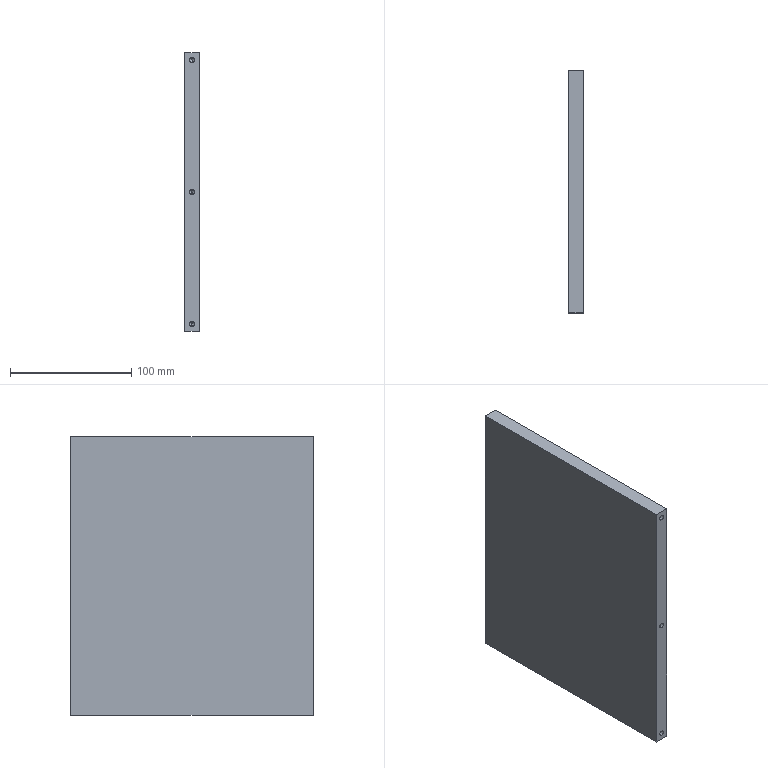Part | SolidWorks | features Extrusion 1, HoleWzd 1, MirrorPattern 1 | 1 solid | 30 faces | box 12 x 200 x 230 mm | volume 549928 mm3 | cylinder 12 | cone 12 | plane 6 | commonest cylinder face diameters 4.2 x12
STEP:
#1=CARTESIAN_POINT('',(0.,-75.5,-106.9));
#2=VERTEX_POINT('',#1);
#3=CARTESIAN_POINT('',(0.,-75.5,-111.1));
#4=VERTEX_POINT('',#3);
#5=CARTESIAN_POINT('',(0.,-75.5,-109.));
#6=DIRECTION('',(0.,-1.,0.));
#7=DIRECTION('',(0.,0.,-1.));
#8=AXIS2_PLACEMENT_3D('',#5,#6,#7);
#9=CIRCLE('',#8,2.1);
#10=EDGE_CURVE('',#2,#4,#9,.T.);
#11=ORIENTED_EDGE('',*,*,#10,.F.);
#12=CARTESIAN_POINT('',(0.,-100.,-106.9));
#13=VERTEX_POINT('',#12);
#14=CARTESIAN_POINT('',(0.,-100.,-106.9));
#15=DIRECTION('',(0.,-1.,0.));
#16=VECTOR('',#15,1000.);
#17=LINE('',#14,#16);
#18=EDGE_CURVE('',#2,#13,#17,.T.);
#19=ORIENTED_EDGE('',*,*,#18,.T.);
#20=CARTESIAN_POINT('',(0.,-100.,-111.1));
#21=VERTEX_POINT('',#20);
#22=CARTESIAN_POINT('',(0.,-100.,-109.));
#23=DIRECTION('',(0.,-1.,0.));
#24=DIRECTION('',(0.,0.,-1.));
#25=AXIS2_PLACEMENT_3D('',#22,#23,#24);
#26=CIRCLE('',#25,2.1);
#27=EDGE_CURVE('',#13,#21,#26,.T.);
#28=ORIENTED_EDGE('',*,*,#27,.T.);
#29=CARTESIAN_POINT('',(0.,-100.,-111.1));
#30=DIRECTION('',(0.,-1.,0.));
#31=VECTOR('',#30,1000.);
#32=LINE('',#29,#31);
#33=EDGE_CURVE('',#4,#21,#32,.T.);
#34=ORIENTED_EDGE('',*,*,#33,.F.);
#35=EDGE_LOOP('',(#11,#19,#28,#34));
#36=FACE_OUTER_BOUND('',#35,.T.);
#37=CARTESIAN_POINT('',(0.,-100.,-109.));
#38=DIRECTION('',(0.,-1.,0.));
#39=DIRECTION('',(0.,0.,-1.));
#40=AXIS2_PLACEMENT_3D('',#37,#38,#39);
#41=CYLINDRICAL_SURFACE('',#40,2.1);
#42=ADVANCED_FACE('',(#36),#41,.F.);
#43=CARTESIAN_POINT('',(0.,-74.238,-109.));
#44=VERTEX_POINT('',#43);
#45=CARTESIAN_POINT('',(0.,-75.5,-111.1));
#46=DIRECTION('',(0.,-0.515,-0.8572));
#47=VECTOR('',#46,1000.);
#48=LINE('',#45,#47);
#49=EDGE_CURVE('',#44,#4,#48,.T.);
#50=ORIENTED_EDGE('',*,*,#49,.F.);
#51=CARTESIAN_POINT('',(0.,-75.5,-106.9));
#52=DIRECTION('',(0.,-0.515,0.8572));
#53=VECTOR('',#52,1000.);
#54=LINE('',#51,#53);
#55=EDGE_CURVE('',#44,#2,#54,.T.);
#56=ORIENTED_EDGE('',*,*,#55,.T.);
#57=ORIENTED_EDGE('',*,*,#10,.T.);
#58=EDGE_LOOP('',(#50,#56,#57));
#59=FACE_OUTER_BOUND('',#58,.T.);
#60=CARTESIAN_POINT('',(0.,-75.5,-109.));
#61=DIRECTION('',(0.,-1.,0.));
#62=DIRECTION('',(0.,0.,-1.));
#63=AXIS2_PLACEMENT_3D('',#60,#61,#62);
#64=CONICAL_SURFACE('',#63,2.1,1.03);
#65=ADVANCED_FACE('',(#59),#64,.F.);
#66=CARTESIAN_POINT('',(0.,-75.5,2.1));
#67=VERTEX_POINT('',#66);
#68=CARTESIAN_POINT('',(0.,-75.5,-2.1));
#69=VERTEX_POINT('',#68);
#70=CARTESIAN_POINT('',(0.,-75.5,0.));
#71=DIRECTION('',(0.,-1.,0.));
#72=DIRECTION('',(0.,0.,-1.));
#73=AXIS2_PLACEMENT_3D('',#70,#71,#72);
#74=CIRCLE('',#73,2.1);
#75=EDGE_CURVE('',#67,#69,#74,.T.);
#76=ORIENTED_EDGE('',*,*,#75,.F.);
#77=CARTESIAN_POINT('',(0.,-100.,2.1));
#78=VERTEX_POINT('',#77);
#79=CARTESIAN_POINT('',(0.,-100.,2.1));
#80=DIRECTION('',(0.,-1.,0.));
#81=VECTOR('',#80,1000.);
#82=LINE('',#79,#81);
#83=EDGE_CURVE('',#67,#78,#82,.T.);
#84=ORIENTED_EDGE('',*,*,#83,.T.);
#85=CARTESIAN_POINT('',(0.,-100.,-2.1));
#86=VERTEX_POINT('',#85);
#87=CARTESIAN_POINT('',(0.,-100.,0.));
#88=DIRECTION('',(0.,-1.,0.));
#89=DIRECTION('',(0.,0.,-1.));
#90=AXIS2_PLACEMENT_3D('',#87,#88,#89);
#91=CIRCLE('',#90,2.1);
#92=EDGE_CURVE('',#78,#86,#91,.T.);
#93=ORIENTED_EDGE('',*,*,#92,.T.);
#94=CARTESIAN_POINT('',(0.,-100.,-2.1));
#95=DIRECTION('',(0.,-1.,0.));
#96=VECTOR('',#95,1000.);
#97=LINE('',#94,#96);
#98=EDGE_CURVE('',#69,#86,#97,.T.);
#99=ORIENTED_EDGE('',*,*,#98,.F.);
#100=EDGE_LOOP('',(#76,#84,#93,#99));
#101=FACE_OUTER_BOUND('',#100,.T.);
#102=CARTESIAN_POINT('',(0.,-100.,0.));
#103=DIRECTION('',(0.,-1.,0.));
#104=DIRECTION('',(0.,0.,-1.));
#105=AXIS2_PLACEMENT_3D('',#102,#103,#104);
#106=CYLINDRICAL_SURFACE('',#105,2.1);
#107=ADVANCED_FACE('',(#101),#106,.F.);
#108=CARTESIAN_POINT('',(0.,-74.238,0.));
#109=VERTEX_POINT('',#108);
#110=CARTESIAN_POINT('',(0.,-75.5,-2.1));
#111=DIRECTION('',(0.,-0.515,-0.8572));
#112=VECTOR('',#111,1000.);
#113=LINE('',#110,#112);
#114=EDGE_CURVE('',#109,#69,#113,.T.);
#115=ORIENTED_EDGE('',*,*,#114,.F.);
#116=CARTESIAN_POINT('',(0.,-75.5,2.1));
#117=DIRECTION('',(0.,-0.515,0.8572));
#118=VECTOR('',#117,1000.);
#119=LINE('',#116,#118);
#120=EDGE_CURVE('',#109,#67,#119,.T.);
#121=ORIENTED_EDGE('',*,*,#120,.T.);
#122=ORIENTED_EDGE('',*,*,#75,.T.);
#123=EDGE_LOOP('',(#115,#121,#122));
#124=FACE_OUTER_BOUND('',#123,.T.);
#125=CARTESIAN_POINT('',(0.,-75.5,0.));
#126=DIRECTION('',(0.,-1.,0.));
#127=DIRECTION('',(0.,0.,-1.));
#128=AXIS2_PLACEMENT_3D('',#125,#126,#127);
#129=CONICAL_SURFACE('',#128,2.1,1.03);
#130=ADVANCED_FACE('',(#124),#129,.F.);
#131=CARTESIAN_POINT('',(0.,-75.5,111.1));
#132=VERTEX_POINT('',#131);
#133=CARTESIAN_POINT('',(0.,-75.5,106.9));
#134=VERTEX_POINT('',#133);
#135=CARTESIAN_POINT('',(0.,-75.5,109.));
#136=DIRECTION('',(0.,-1.,0.));
#137=DIRECTION('',(0.,0.,-1.));
#138=AXIS2_PLACEMENT_3D('',#135,#136,#137);
#139=CIRCLE('',#138,2.1);
#140=EDGE_CURVE('',#132,#134,#139,.T.);
#141=ORIENTED_EDGE('',*,*,#140,.F.);
#142=CARTESIAN_POINT('',(0.,-100.,111.1));
#143=VERTEX_POINT('',#142);
#144=CARTESIAN_POINT('',(0.,-100.,111.1));
#145=DIRECTION('',(0.,-1.,0.));
#146=VECTOR('',#145,1000.);
#147=LINE('',#144,#146);
#148=EDGE_CURVE('',#132,#143,#147,.T.);
#149=ORIENTED_EDGE('',*,*,#148,.T.);
#150=CARTESIAN_POINT('',(0.,-100.,106.9));
#151=VERTEX_POINT('',#150);
#152=CARTESIAN_POINT('',(0.,-100.,109.));
#153=DIRECTION('',(0.,-1.,0.));
#154=DIRECTION('',(0.,0.,-1.));
#155=AXIS2_PLACEMENT_3D('',#152,#153,#154);
#156=CIRCLE('',#155,2.1);
#157=EDGE_CURVE('',#143,#151,#156,.T.);
#158=ORIENTED_EDGE('',*,*,#157,.T.);
#159=CARTESIAN_POINT('',(0.,-100.,106.9));
#160=DIRECTION('',(0.,-1.,0.));
#161=VECTOR('',#160,1000.);
#162=LINE('',#159,#161);
#163=EDGE_CURVE('',#134,#151,#162,.T.);
#164=ORIENTED_EDGE('',*,*,#163,.F.);
#165=EDGE_LOOP('',(#141,#149,#158,#164));
#166=FACE_OUTER_BOUND('',#165,.T.);
#167=CARTESIAN_POINT('',(0.,-100.,109.));
#168=DIRECTION('',(0.,-1.,0.));
#169=DIRECTION('',(0.,0.,-1.));
#170=AXIS2_PLACEMENT_3D('',#167,#168,#169);
#171=CYLINDRICAL_SURFACE('',#170,2.1);
#172=ADVANCED_FACE('',(#166),#171,.F.);
#173=CARTESIAN_POINT('',(0.,-74.238,109.));
#174=VERTEX_POINT('',#173);
#175=CARTESIAN_POINT('',(0.,-75.5,106.9));
#176=DIRECTION('',(0.,-0.515,-0.8572));
#177=VECTOR('',#176,1000.);
#178=LINE('',#175,#177);
#179=EDGE_CURVE('',#174,#134,#178,.T.);
#180=ORIENTED_EDGE('',*,*,#179,.F.);
#181=CARTESIAN_POINT('',(0.,-75.5,111.1));
#182=DIRECTION('',(0.,-0.515,0.8572));
#183=VECTOR('',#182,1000.);
#184=LINE('',#181,#183);
#185=EDGE_CURVE('',#174,#132,#184,.T.);
#186=ORIENTED_EDGE('',*,*,#185,.T.);
#187=ORIENTED_EDGE('',*,*,#140,.T.);
#188=EDGE_LOOP('',(#180,#186,#187));
#189=FACE_OUTER_BOUND('',#188,.T.);
#190=CARTESIAN_POINT('',(0.,-75.5,109.));
#191=DIRECTION('',(0.,-1.,0.));
#192=DIRECTION('',(0.,0.,-1.));
#193=AXIS2_PLACEMENT_3D('',#190,#191,#192);
#194=CONICAL_SURFACE('',#193,2.1,1.03);
#195=ADVANCED_FACE('',(#189),#194,.F.);
#196=CARTESIAN_POINT('',(0.,75.5,-111.1));
#197=VERTEX_POINT('',#196);
#198=CARTESIAN_POINT('',(0.,75.5,-106.9));
#199=VERTEX_POINT('',#198);
#200=CARTESIAN_POINT('',(0.,75.5,-109.));
#201=DIRECTION('',(0.,1.,0.));
#202=DIRECTION('',(0.,0.,1.));
#203=AXIS2_PLACEMENT_3D('',#200,#201,#202);
#204=CIRCLE('',#203,2.1);
#205=EDGE_CURVE('',#197,#199,#204,.T.);
#206=ORIENTED_EDGE('',*,*,#205,.F.);
#207=CARTESIAN_POINT('',(0.,100.,-111.1));
#208=VERTEX_POINT('',#207);
#209=CARTESIAN_POINT('',(0.,100.,-111.1));
#210=DIRECTION('',(0.,1.,0.));
#211=VECTOR('',#210,1000.);
#212=LINE('',#209,#211);
#213=EDGE_CURVE('',#197,#208,#212,.T.);
#214=ORIENTED_EDGE('',*,*,#213,.T.);
#215=CARTESIAN_POINT('',(0.,100.,-106.9));
#216=VERTEX_POINT('',#215);
#217=CARTESIAN_POINT('',(0.,100.,-109.));
#218=DIRECTION('',(0.,1.,0.));
#219=DIRECTION('',(0.,0.,1.));
#220=AXIS2_PLACEMENT_3D('',#217,#218,#219);
#221=CIRCLE('',#220,2.1);
#222=EDGE_CURVE('',#208,#216,#221,.T.);
#223=ORIENTED_EDGE('',*,*,#222,.T.);
#224=CARTESIAN_POINT('',(0.,100.,-106.9));
#225=DIRECTION('',(0.,1.,0.));
#226=VECTOR('',#225,1000.);
#227=LINE('',#224,#226);
#228=EDGE_CURVE('',#199,#216,#227,.T.);
#229=ORIENTED_EDGE('',*,*,#228,.F.);
#230=EDGE_LOOP('',(#206,#214,#223,#229));
#231=FACE_OUTER_BOUND('',#230,.T.);
#232=CARTESIAN_POINT('',(0.,100.,-109.));
#233=DIRECTION('',(0.,1.,0.));
#234=DIRECTION('',(0.,0.,1.));
#235=AXIS2_PLACEMENT_3D('',#232,#233,#234);
#236=CYLINDRICAL_SURFACE('',#235,2.1);
#237=ADVANCED_FACE('',(#231),#236,.F.);
#238=CARTESIAN_POINT('',(0.,74.238,-109.));
#239=VERTEX_POINT('',#238);
#240=CARTESIAN_POINT('',(0.,75.5,-106.9));
#241=DIRECTION('',(0.,0.515,0.8572));
#242=VECTOR('',#241,1000.);
#243=LINE('',#240,#242);
#244=EDGE_CURVE('',#239,#199,#243,.T.);
#245=ORIENTED_EDGE('',*,*,#244,.F.);
#246=CARTESIAN_POINT('',(0.,75.5,-111.1));
#247=DIRECTION('',(0.,0.515,-0.8572));
#248=VECTOR('',#247,1000.);
#249=LINE('',#246,#248);
#250=EDGE_CURVE('',#239,#197,#249,.T.);
#251=ORIENTED_EDGE('',*,*,#250,.T.);
#252=ORIENTED_EDGE('',*,*,#205,.T.);
#253=EDGE_LOOP('',(#245,#251,#252));
#254=FACE_OUTER_BOUND('',#253,.T.);
#255=CARTESIAN_POINT('',(0.,75.5,-109.));
#256=DIRECTION('',(0.,1.,0.));
#257=DIRECTION('',(0.,0.,1.));
#258=AXIS2_PLACEMENT_3D('',#255,#256,#257);
#259=CONICAL_SURFACE('',#258,2.1,1.03);
#260=ADVANCED_FACE('',(#254),#259,.F.);
#261=CARTESIAN_POINT('',(0.,75.5,-2.1));
#262=VERTEX_POINT('',#261);
#263=CARTESIAN_POINT('',(0.,75.5,2.1));
#264=VERTEX_POINT('',#263);
#265=CARTESIAN_POINT('',(0.,75.5,0.));
#266=DIRECTION('',(0.,1.,0.));
#267=DIRECTION('',(0.,0.,1.));
#268=AXIS2_PLACEMENT_3D('',#265,#266,#267);
#269=CIRCLE('',#268,2.1);
#270=EDGE_CURVE('',#262,#264,#269,.T.);
#271=ORIENTED_EDGE('',*,*,#270,.F.);
#272=CARTESIAN_POINT('',(0.,100.,-2.1));
#273=VERTEX_POINT('',#272);
#274=CARTESIAN_POINT('',(0.,100.,-2.1));
#275=DIRECTION('',(0.,1.,0.));
#276=VECTOR('',#275,1000.);
#277=LINE('',#274,#276);
#278=EDGE_CURVE('',#262,#273,#277,.T.);
#279=ORIENTED_EDGE('',*,*,#278,.T.);
#280=CARTESIAN_POINT('',(0.,100.,2.1));
#281=VERTEX_POINT('',#280);
#282=CARTESIAN_POINT('',(0.,100.,0.));
#283=DIRECTION('',(0.,1.,0.));
#284=DIRECTION('',(0.,0.,1.));
#285=AXIS2_PLACEMENT_3D('',#282,#283,#284);
#286=CIRCLE('',#285,2.1);
#287=EDGE_CURVE('',#273,#281,#286,.T.);
#288=ORIENTED_EDGE('',*,*,#287,.T.);
#289=CARTESIAN_POINT('',(0.,100.,2.1));
#290=DIRECTION('',(0.,1.,0.));
#291=VECTOR('',#290,1000.);
#292=LINE('',#289,#291);
#293=EDGE_CURVE('',#264,#281,#292,.T.);
#294=ORIENTED_EDGE('',*,*,#293,.F.);
#295=EDGE_LOOP('',(#271,#279,#288,#294));
#296=FACE_OUTER_BOUND('',#295,.T.);
#297=CARTESIAN_POINT('',(0.,100.,0.));
#298=DIRECTION('',(0.,1.,0.));
#299=DIRECTION('',(0.,0.,1.));
#300=AXIS2_PLACEMENT_3D('',#297,#298,#299);
#301=CYLINDRICAL_SURFACE('',#300,2.1);
#302=ADVANCED_FACE('',(#296),#301,.F.);
#303=CARTESIAN_POINT('',(0.,74.238,0.));
#304=VERTEX_POINT('',#303);
#305=CARTESIAN_POINT('',(0.,75.5,2.1));
#306=DIRECTION('',(0.,0.515,0.8572));
#307=VECTOR('',#306,1000.);
#308=LINE('',#305,#307);
#309=EDGE_CURVE('',#304,#264,#308,.T.);
#310=ORIENTED_EDGE('',*,*,#309,.F.);
#311=CARTESIAN_POINT('',(0.,75.5,-2.1));
#312=DIRECTION('',(0.,0.515,-0.8572));
#313=VECTOR('',#312,1000.);
#314=LINE('',#311,#313);
#315=EDGE_CURVE('',#304,#262,#314,.T.);
#316=ORIENTED_EDGE('',*,*,#315,.T.);
#317=ORIENTED_EDGE('',*,*,#270,.T.);
#318=EDGE_LOOP('',(#310,#316,#317));
#319=FACE_OUTER_BOUND('',#318,.T.);
#320=CARTESIAN_POINT('',(0.,75.5,0.));
#321=DIRECTION('',(0.,1.,0.));
#322=DIRECTION('',(0.,0.,1.));
#323=AXIS2_PLACEMENT_3D('',#320,#321,#322);
#324=CONICAL_SURFACE('',#323,2.1,1.03);
#325=ADVANCED_FACE('',(#319),#324,.F.);
#326=CARTESIAN_POINT('',(0.,75.5,106.9));
#327=VERTEX_POINT('',#326);
#328=CARTESIAN_POINT('',(0.,75.5,111.1));
#329=VERTEX_POINT('',#328);
#330=CARTESIAN_POINT('',(0.,75.5,109.));
#331=DIRECTION('',(0.,1.,0.));
#332=DIRECTION('',(0.,0.,1.));
#333=AXIS2_PLACEMENT_3D('',#330,#331,#332);
#334=CIRCLE('',#333,2.1);
#335=EDGE_CURVE('',#327,#329,#334,.T.);
#336=ORIENTED_EDGE('',*,*,#335,.F.);
#337=CARTESIAN_POINT('',(0.,100.,106.9));
#338=VERTEX_POINT('',#337);
#339=CARTESIAN_POINT('',(0.,100.,106.9));
#340=DIRECTION('',(0.,1.,0.));
#341=VECTOR('',#340,1000.);
#342=LINE('',#339,#341);
#343=EDGE_CURVE('',#327,#338,#342,.T.);
#344=ORIENTED_EDGE('',*,*,#343,.T.);
#345=CARTESIAN_POINT('',(0.,100.,111.1));
#346=VERTEX_POINT('',#345);
#347=CARTESIAN_POINT('',(0.,100.,109.));
#348=DIRECTION('',(0.,1.,0.));
#349=DIRECTION('',(0.,0.,1.));
#350=AXIS2_PLACEMENT_3D('',#347,#348,#349);
#351=CIRCLE('',#350,2.1);
#352=EDGE_CURVE('',#338,#346,#351,.T.);
#353=ORIENTED_EDGE('',*,*,#352,.T.);
#354=CARTESIAN_POINT('',(0.,100.,111.1));
#355=DIRECTION('',(0.,1.,0.));
#356=VECTOR('',#355,1000.);
#357=LINE('',#354,#356);
#358=EDGE_CURVE('',#329,#346,#357,.T.);
#359=ORIENTED_EDGE('',*,*,#358,.F.);
#360=EDGE_LOOP('',(#336,#344,#353,#359));
#361=FACE_OUTER_BOUND('',#360,.T.);
#362=CARTESIAN_POINT('',(0.,100.,109.));
#363=DIRECTION('',(0.,1.,0.));
#364=DIRECTION('',(0.,0.,1.));
#365=AXIS2_PLACEMENT_3D('',#362,#363,#364);
#366=CYLINDRICAL_SURFACE('',#365,2.1);
#367=ADVANCED_FACE('',(#361),#366,.F.);
#368=CARTESIAN_POINT('',(0.,74.238,109.));
#369=VERTEX_POINT('',#368);
#370=CARTESIAN_POINT('',(0.,75.5,111.1));
#371=DIRECTION('',(0.,0.515,0.8572));
#372=VECTOR('',#371,1000.);
#373=LINE('',#370,#372);
#374=EDGE_CURVE('',#369,#329,#373,.T.);
#375=ORIENTED_EDGE('',*,*,#374,.F.);
#376=CARTESIAN_POINT('',(0.,75.5,106.9));
#377=DIRECTION('',(0.,0.515,-0.8572));
#378=VECTOR('',#377,1000.);
#379=LINE('',#376,#378);
#380=EDGE_CURVE('',#369,#327,#379,.T.);
#381=ORIENTED_EDGE('',*,*,#380,.T.);
#382=ORIENTED_EDGE('',*,*,#335,.T.);
#383=EDGE_LOOP('',(#375,#381,#382));
#384=FACE_OUTER_BOUND('',#383,.T.);
#385=CARTESIAN_POINT('',(0.,75.5,109.));
#386=DIRECTION('',(0.,1.,0.));
#387=DIRECTION('',(0.,0.,1.));
#388=AXIS2_PLACEMENT_3D('',#385,#386,#387);
#389=CONICAL_SURFACE('',#388,2.1,1.03);
#390=ADVANCED_FACE('',(#384),#389,.F.);
#391=CARTESIAN_POINT('',(-6.,-100.,-115.));
#392=VERTEX_POINT('',#391);
#393=CARTESIAN_POINT('',(-6.,100.,-115.));
#394=VERTEX_POINT('',#393);
#395=CARTESIAN_POINT('',(-6.,100.,-115.));
#396=DIRECTION('',(0.,1.,0.));
#397=VECTOR('',#396,1000.);
#398=LINE('',#395,#397);
#399=EDGE_CURVE('',#392,#394,#398,.T.);
#400=ORIENTED_EDGE('',*,*,#399,.T.);
#401=CARTESIAN_POINT('',(6.,100.,-115.));
#402=VERTEX_POINT('',#401);
#403=CARTESIAN_POINT('',(6.,100.,-115.));
#404=DIRECTION('',(-1.,0.,0.));
#405=VECTOR('',#404,1000.);
#406=LINE('',#403,#405);
#407=EDGE_CURVE('',#402,#394,#406,.T.);
#408=ORIENTED_EDGE('',*,*,#407,.F.);
#409=CARTESIAN_POINT('',(6.,-100.,-115.));
#410=VERTEX_POINT('',#409);
#411=CARTESIAN_POINT('',(6.,100.,-115.));
#412=DIRECTION('',(0.,1.,0.));
#413=VECTOR('',#412,1000.);
#414=LINE('',#411,#413);
#415=EDGE_CURVE('',#410,#402,#414,.T.);
#416=ORIENTED_EDGE('',*,*,#415,.F.);
#417=CARTESIAN_POINT('',(6.,-100.,-115.));
#418=DIRECTION('',(-1.,0.,0.));
#419=VECTOR('',#418,1000.);
#420=LINE('',#417,#419);
#421=EDGE_CURVE('',#410,#392,#420,.T.);
#422=ORIENTED_EDGE('',*,*,#421,.T.);
#423=EDGE_LOOP('',(#400,#408,#416,#422));
#424=FACE_OUTER_BOUND('',#423,.T.);
#425=CARTESIAN_POINT('',(6.,100.,-115.));
#426=DIRECTION('',(0.,0.,1.));
#427=DIRECTION('',(0.,-1.,0.));
#428=AXIS2_PLACEMENT_3D('',#425,#426,#427);
#429=PLANE('',#428);
#430=ADVANCED_FACE('',(#424),#429,.F.);
#431=CARTESIAN_POINT('',(0.,100.,-109.));
#432=DIRECTION('',(0.,1.,0.));
#433=DIRECTION('',(0.,0.,1.));
#434=AXIS2_PLACEMENT_3D('',#431,#432,#433);
#435=CIRCLE('',#434,2.1);
#436=EDGE_CURVE('',#216,#208,#435,.T.);
#437=ORIENTED_EDGE('',*,*,#436,.F.);
#438=ORIENTED_EDGE('',*,*,#222,.F.);
#439=EDGE_LOOP('',(#437,#438));
#440=FACE_BOUND('',#439,.T.);
#441=CARTESIAN_POINT('',(0.,100.,0.));
#442=DIRECTION('',(0.,1.,0.));
#443=DIRECTION('',(0.,0.,1.));
#444=AXIS2_PLACEMENT_3D('',#441,#442,#443);
#445=CIRCLE('',#444,2.1);
#446=EDGE_CURVE('',#281,#273,#445,.T.);
#447=ORIENTED_EDGE('',*,*,#446,.F.);
#448=ORIENTED_EDGE('',*,*,#287,.F.);
#449=EDGE_LOOP('',(#447,#448));
#450=FACE_BOUND('',#449,.T.);
#451=CARTESIAN_POINT('',(0.,100.,109.));
#452=DIRECTION('',(0.,1.,0.));
#453=DIRECTION('',(0.,0.,1.));
#454=AXIS2_PLACEMENT_3D('',#451,#452,#453);
#455=CIRCLE('',#454,2.1);
#456=EDGE_CURVE('',#346,#338,#455,.T.);
#457=ORIENTED_EDGE('',*,*,#456,.F.);
#458=ORIENTED_EDGE('',*,*,#352,.F.);
#459=EDGE_LOOP('',(#457,#458));
#460=FACE_BOUND('',#459,.T.);
#461=CARTESIAN_POINT('',(-6.,100.,115.));
#462=VERTEX_POINT('',#461);
#463=CARTESIAN_POINT('',(-6.,100.,115.));
#464=DIRECTION('',(0.,0.,1.));
#465=VECTOR('',#464,1000.);
#466=LINE('',#463,#465);
#467=EDGE_CURVE('',#394,#462,#466,.T.);
#468=ORIENTED_EDGE('',*,*,#467,.T.);
#469=CARTESIAN_POINT('',(6.,100.,115.));
#470=VERTEX_POINT('',#469);
#471=CARTESIAN_POINT('',(6.,100.,115.));
#472=DIRECTION('',(-1.,0.,0.));
#473=VECTOR('',#472,1000.);
#474=LINE('',#471,#473);
#475=EDGE_CURVE('',#470,#462,#474,.T.);
#476=ORIENTED_EDGE('',*,*,#475,.F.);
#477=CARTESIAN_POINT('',(6.,100.,115.));
#478=DIRECTION('',(0.,0.,1.));
#479=VECTOR('',#478,1000.);
#480=LINE('',#477,#479);
#481=EDGE_CURVE('',#402,#470,#480,.T.);
#482=ORIENTED_EDGE('',*,*,#481,.F.);
#483=ORIENTED_EDGE('',*,*,#407,.T.);
#484=EDGE_LOOP('',(#468,#476,#482,#483));
#485=FACE_OUTER_BOUND('',#484,.T.);
#486=CARTESIAN_POINT('',(6.,100.,115.));
#487=DIRECTION('',(0.,-1.,0.));
#488=DIRECTION('',(0.,0.,-1.));
#489=AXIS2_PLACEMENT_3D('',#486,#487,#488);
#490=PLANE('',#489);
#491=ADVANCED_FACE('',(#440,#450,#460,#485),#490,.F.);
#492=CARTESIAN_POINT('',(-6.,-100.,115.));
#493=VERTEX_POINT('',#492);
#494=CARTESIAN_POINT('',(-6.,100.,115.));
#495=DIRECTION('',(0.,-1.,0.));
#496=VECTOR('',#495,1000.);
#497=LINE('',#494,#496);
#498=EDGE_CURVE('',#462,#493,#497,.T.);
#499=ORIENTED_EDGE('',*,*,#498,.T.);
#500=CARTESIAN_POINT('',(6.,-100.,115.));
#501=VERTEX_POINT('',#500);
#502=CARTESIAN_POINT('',(6.,-100.,115.));
#503=DIRECTION('',(-1.,0.,0.));
#504=VECTOR('',#503,1000.);
#505=LINE('',#502,#504);
#506=EDGE_CURVE('',#501,#493,#505,.T.);
#507=ORIENTED_EDGE('',*,*,#506,.F.);
#508=CARTESIAN_POINT('',(6.,100.,115.));
#509=DIRECTION('',(0.,-1.,0.));
#510=VECTOR('',#509,1000.);
#511=LINE('',#508,#510);
#512=EDGE_CURVE('',#470,#501,#511,.T.);
#513=ORIENTED_EDGE('',*,*,#512,.F.);
#514=ORIENTED_EDGE('',*,*,#475,.T.);
#515=EDGE_LOOP('',(#499,#507,#513,#514));
#516=FACE_OUTER_BOUND('',#515,.T.);
#517=CARTESIAN_POINT('',(6.,100.,115.));
#518=DIRECTION('',(0.,0.,-1.));
#519=DIRECTION('',(0.,1.,0.));
#520=AXIS2_PLACEMENT_3D('',#517,#518,#519);
#521=PLANE('',#520);
#522=ADVANCED_FACE('',(#516),#521,.F.);
#523=CARTESIAN_POINT('',(0.,-100.,-109.));
#524=DIRECTION('',(0.,-1.,0.));
#525=DIRECTION('',(0.,0.,-1.));
#526=AXIS2_PLACEMENT_3D('',#523,#524,#525);
#527=CIRCLE('',#526,2.1);
#528=EDGE_CURVE('',#21,#13,#527,.T.);
#529=ORIENTED_EDGE('',*,*,#528,.F.);
#530=ORIENTED_EDGE('',*,*,#27,.F.);
#531=EDGE_LOOP('',(#529,#530));
#532=FACE_BOUND('',#531,.T.);
#533=CARTESIAN_POINT('',(0.,-100.,0.));
#534=DIRECTION('',(0.,-1.,0.));
#535=DIRECTION('',(0.,0.,-1.));
#536=AXIS2_PLACEMENT_3D('',#533,#534,#535);
#537=CIRCLE('',#536,2.1);
#538=EDGE_CURVE('',#86,#78,#537,.T.);
#539=ORIENTED_EDGE('',*,*,#538,.F.);
#540=ORIENTED_EDGE('',*,*,#92,.F.);
#541=EDGE_LOOP('',(#539,#540));
#542=FACE_BOUND('',#541,.T.);
#543=CARTESIAN_POINT('',(0.,-100.,109.));
#544=DIRECTION('',(0.,-1.,0.));
#545=DIRECTION('',(0.,0.,-1.));
#546=AXIS2_PLACEMENT_3D('',#543,#544,#545);
#547=CIRCLE('',#546,2.1);
#548=EDGE_CURVE('',#151,#143,#547,.T.);
#549=ORIENTED_EDGE('',*,*,#548,.F.);
#550=ORIENTED_EDGE('',*,*,#157,.F.);
#551=EDGE_LOOP('',(#549,#550));
#552=FACE_BOUND('',#551,.T.);
#553=CARTESIAN_POINT('',(-6.,-100.,115.));
#554=DIRECTION('',(0.,0.,-1.));
#555=VECTOR('',#554,1000.);
#556=LINE('',#553,#555);
#557=EDGE_CURVE('',#493,#392,#556,.T.);
#558=ORIENTED_EDGE('',*,*,#557,.T.);
#559=ORIENTED_EDGE('',*,*,#421,.F.);
#560=CARTESIAN_POINT('',(6.,-100.,115.));
#561=DIRECTION('',(0.,0.,-1.));
#562=VECTOR('',#561,1000.);
#563=LINE('',#560,#562);
#564=EDGE_CURVE('',#501,#410,#563,.T.);
#565=ORIENTED_EDGE('',*,*,#564,.F.);
#566=ORIENTED_EDGE('',*,*,#506,.T.);
#567=EDGE_LOOP('',(#558,#559,#565,#566));
#568=FACE_OUTER_BOUND('',#567,.T.);
#569=CARTESIAN_POINT('',(6.,-100.,115.));
#570=DIRECTION('',(0.,1.,0.));
#571=DIRECTION('',(0.,0.,1.));
#572=AXIS2_PLACEMENT_3D('',#569,#570,#571);
#573=PLANE('',#572);
#574=ADVANCED_FACE('',(#532,#542,#552,#568),#573,.F.);
#575=ORIENTED_EDGE('',*,*,#415,.T.);
#576=ORIENTED_EDGE('',*,*,#481,.T.);
#577=ORIENTED_EDGE('',*,*,#512,.T.);
#578=ORIENTED_EDGE('',*,*,#564,.T.);
#579=EDGE_LOOP('',(#575,#576,#577,#578));
#580=FACE_OUTER_BOUND('',#579,.T.);
#581=CARTESIAN_POINT('',(6.,0.,0.));
#582=DIRECTION('',(1.,0.,0.));
#583=DIRECTION('',(0.,0.,-1.));
#584=AXIS2_PLACEMENT_3D('',#581,#582,#583);
#585=PLANE('',#584);
#586=ADVANCED_FACE('',(#580),#585,.T.);
#587=ORIENTED_EDGE('',*,*,#399,.F.);
#588=ORIENTED_EDGE('',*,*,#557,.F.);
#589=ORIENTED_EDGE('',*,*,#498,.F.);
#590=ORIENTED_EDGE('',*,*,#467,.F.);
#591=EDGE_LOOP('',(#587,#588,#589,#590));
#592=FACE_OUTER_BOUND('',#591,.T.);
#593=CARTESIAN_POINT('',(-6.,0.,0.));
#594=DIRECTION('',(1.,0.,0.));
#595=DIRECTION('',(0.,0.,-1.));
#596=AXIS2_PLACEMENT_3D('',#593,#594,#595);
#597=PLANE('',#596);
#598=ADVANCED_FACE('',(#592),#597,.F.);
#599=ORIENTED_EDGE('',*,*,#380,.F.);
#600=ORIENTED_EDGE('',*,*,#374,.T.);
#601=CARTESIAN_POINT('',(0.,75.5,109.));
#602=DIRECTION('',(0.,1.,0.));
#603=DIRECTION('',(0.,0.,1.));
#604=AXIS2_PLACEMENT_3D('',#601,#602,#603);
#605=CIRCLE('',#604,2.1);
#606=EDGE_CURVE('',#329,#327,#605,.T.);
#607=ORIENTED_EDGE('',*,*,#606,.T.);
#608=EDGE_LOOP('',(#599,#600,#607));
#609=FACE_OUTER_BOUND('',#608,.T.);
#610=CARTESIAN_POINT('',(0.,75.5,109.));
#611=DIRECTION('',(0.,1.,0.));
#612=DIRECTION('',(0.,0.,1.));
#613=AXIS2_PLACEMENT_3D('',#610,#611,#612);
#614=CONICAL_SURFACE('',#613,2.1,1.03);
#615=ADVANCED_FACE('',(#609),#614,.F.);
#616=ORIENTED_EDGE('',*,*,#343,.F.);
#617=ORIENTED_EDGE('',*,*,#606,.F.);
#618=ORIENTED_EDGE('',*,*,#358,.T.);
#619=ORIENTED_EDGE('',*,*,#456,.T.);
#620=EDGE_LOOP('',(#616,#617,#618,#619));
#621=FACE_OUTER_BOUND('',#620,.T.);
#622=CARTESIAN_POINT('',(0.,100.,109.));
#623=DIRECTION('',(0.,1.,0.));
#624=DIRECTION('',(0.,0.,1.));
#625=AXIS2_PLACEMENT_3D('',#622,#623,#624);
#626=CYLINDRICAL_SURFACE('',#625,2.1);
#627=ADVANCED_FACE('',(#621),#626,.F.);
#628=ORIENTED_EDGE('',*,*,#315,.F.);
#629=ORIENTED_EDGE('',*,*,#309,.T.);
#630=CARTESIAN_POINT('',(0.,75.5,0.));
#631=DIRECTION('',(0.,1.,0.));
#632=DIRECTION('',(0.,0.,1.));
#633=AXIS2_PLACEMENT_3D('',#630,#631,#632);
#634=CIRCLE('',#633,2.1);
#635=EDGE_CURVE('',#264,#262,#634,.T.);
#636=ORIENTED_EDGE('',*,*,#635,.T.);
#637=EDGE_LOOP('',(#628,#629,#636));
#638=FACE_OUTER_BOUND('',#637,.T.);
#639=CARTESIAN_POINT('',(0.,75.5,0.));
#640=DIRECTION('',(0.,1.,0.));
#641=DIRECTION('',(0.,0.,1.));
#642=AXIS2_PLACEMENT_3D('',#639,#640,#641);
#643=CONICAL_SURFACE('',#642,2.1,1.03);
#644=ADVANCED_FACE('',(#638),#643,.F.);
#645=ORIENTED_EDGE('',*,*,#278,.F.);
#646=ORIENTED_EDGE('',*,*,#635,.F.);
#647=ORIENTED_EDGE('',*,*,#293,.T.);
#648=ORIENTED_EDGE('',*,*,#446,.T.);
#649=EDGE_LOOP('',(#645,#646,#647,#648));
#650=FACE_OUTER_BOUND('',#649,.T.);
#651=CARTESIAN_POINT('',(0.,100.,0.));
#652=DIRECTION('',(0.,1.,0.));
#653=DIRECTION('',(0.,0.,1.));
#654=AXIS2_PLACEMENT_3D('',#651,#652,#653);
#655=CYLINDRICAL_SURFACE('',#654,2.1);
#656=ADVANCED_FACE('',(#650),#655,.F.);
#657=ORIENTED_EDGE('',*,*,#250,.F.);
#658=ORIENTED_EDGE('',*,*,#244,.T.);
#659=CARTESIAN_POINT('',(0.,75.5,-109.));
#660=DIRECTION('',(0.,1.,0.));
#661=DIRECTION('',(0.,0.,1.));
#662=AXIS2_PLACEMENT_3D('',#659,#660,#661);
#663=CIRCLE('',#662,2.1);
#664=EDGE_CURVE('',#199,#197,#663,.T.);
#665=ORIENTED_EDGE('',*,*,#664,.T.);
#666=EDGE_LOOP('',(#657,#658,#665));
#667=FACE_OUTER_BOUND('',#666,.T.);
#668=CARTESIAN_POINT('',(0.,75.5,-109.));
#669=DIRECTION('',(0.,1.,0.));
#670=DIRECTION('',(0.,0.,1.));
#671=AXIS2_PLACEMENT_3D('',#668,#669,#670);
#672=CONICAL_SURFACE('',#671,2.1,1.03);
#673=ADVANCED_FACE('',(#667),#672,.F.);
#674=ORIENTED_EDGE('',*,*,#213,.F.);
#675=ORIENTED_EDGE('',*,*,#664,.F.);
#676=ORIENTED_EDGE('',*,*,#228,.T.);
#677=ORIENTED_EDGE('',*,*,#436,.T.);
#678=EDGE_LOOP('',(#674,#675,#676,#677));
#679=FACE_OUTER_BOUND('',#678,.T.);
#680=CARTESIAN_POINT('',(0.,100.,-109.));
#681=DIRECTION('',(0.,1.,0.));
#682=DIRECTION('',(0.,0.,1.));
#683=AXIS2_PLACEMENT_3D('',#680,#681,#682);
#684=CYLINDRICAL_SURFACE('',#683,2.1);
#685=ADVANCED_FACE('',(#679),#684,.F.);
#686=ORIENTED_EDGE('',*,*,#185,.F.);
#687=ORIENTED_EDGE('',*,*,#179,.T.);
#688=CARTESIAN_POINT('',(0.,-75.5,109.));
#689=DIRECTION('',(0.,-1.,0.));
#690=DIRECTION('',(0.,0.,-1.));
#691=AXIS2_PLACEMENT_3D('',#688,#689,#690);
#692=CIRCLE('',#691,2.1);
#693=EDGE_CURVE('',#134,#132,#692,.T.);
#694=ORIENTED_EDGE('',*,*,#693,.T.);
#695=EDGE_LOOP('',(#686,#687,#694));
#696=FACE_OUTER_BOUND('',#695,.T.);
#697=CARTESIAN_POINT('',(0.,-75.5,109.));
#698=DIRECTION('',(0.,-1.,0.));
#699=DIRECTION('',(0.,0.,-1.));
#700=AXIS2_PLACEMENT_3D('',#697,#698,#699);
#701=CONICAL_SURFACE('',#700,2.1,1.03);
#702=ADVANCED_FACE('',(#696),#701,.F.);
#703=ORIENTED_EDGE('',*,*,#148,.F.);
#704=ORIENTED_EDGE('',*,*,#693,.F.);
#705=ORIENTED_EDGE('',*,*,#163,.T.);
#706=ORIENTED_EDGE('',*,*,#548,.T.);
#707=EDGE_LOOP('',(#703,#704,#705,#706));
#708=FACE_OUTER_BOUND('',#707,.T.);
#709=CARTESIAN_POINT('',(0.,-100.,109.));
#710=DIRECTION('',(0.,-1.,0.));
#711=DIRECTION('',(0.,0.,-1.));
#712=AXIS2_PLACEMENT_3D('',#709,#710,#711);
#713=CYLINDRICAL_SURFACE('',#712,2.1);
#714=ADVANCED_FACE('',(#708),#713,.F.);
#715=ORIENTED_EDGE('',*,*,#120,.F.);
#716=ORIENTED_EDGE('',*,*,#114,.T.);
#717=CARTESIAN_POINT('',(0.,-75.5,0.));
#718=DIRECTION('',(0.,-1.,0.));
#719=DIRECTION('',(0.,0.,-1.));
#720=AXIS2_PLACEMENT_3D('',#717,#718,#719);
#721=CIRCLE('',#720,2.1);
#722=EDGE_CURVE('',#69,#67,#721,.T.);
#723=ORIENTED_EDGE('',*,*,#722,.T.);
#724=EDGE_LOOP('',(#715,#716,#723));
#725=FACE_OUTER_BOUND('',#724,.T.);
#726=CARTESIAN_POINT('',(0.,-75.5,0.));
#727=DIRECTION('',(0.,-1.,0.));
#728=DIRECTION('',(0.,0.,-1.));
#729=AXIS2_PLACEMENT_3D('',#726,#727,#728);
#730=CONICAL_SURFACE('',#729,2.1,1.03);
#731=ADVANCED_FACE('',(#725),#730,.F.);
#732=ORIENTED_EDGE('',*,*,#83,.F.);
#733=ORIENTED_EDGE('',*,*,#722,.F.);
#734=ORIENTED_EDGE('',*,*,#98,.T.);
#735=ORIENTED_EDGE('',*,*,#538,.T.);
#736=EDGE_LOOP('',(#732,#733,#734,#735));
#737=FACE_OUTER_BOUND('',#736,.T.);
#738=CARTESIAN_POINT('',(0.,-100.,0.));
#739=DIRECTION('',(0.,-1.,0.));
#740=DIRECTION('',(0.,0.,-1.));
#741=AXIS2_PLACEMENT_3D('',#738,#739,#740);
#742=CYLINDRICAL_SURFACE('',#741,2.1);
#743=ADVANCED_FACE('',(#737),#742,.F.);
#744=ORIENTED_EDGE('',*,*,#55,.F.);
#745=ORIENTED_EDGE('',*,*,#49,.T.);
#746=CARTESIAN_POINT('',(0.,-75.5,-109.));
#747=DIRECTION('',(0.,-1.,0.));
#748=DIRECTION('',(0.,0.,-1.));
#749=AXIS2_PLACEMENT_3D('',#746,#747,#748);
#750=CIRCLE('',#749,2.1);
#751=EDGE_CURVE('',#4,#2,#750,.T.);
#752=ORIENTED_EDGE('',*,*,#751,.T.);
#753=EDGE_LOOP('',(#744,#745,#752));
#754=FACE_OUTER_BOUND('',#753,.T.);
#755=CARTESIAN_POINT('',(0.,-75.5,-109.));
#756=DIRECTION('',(0.,-1.,0.));
#757=DIRECTION('',(0.,0.,-1.));
#758=AXIS2_PLACEMENT_3D('',#755,#756,#757);
#759=CONICAL_SURFACE('',#758,2.1,1.03);
#760=ADVANCED_FACE('',(#754),#759,.F.);
#761=ORIENTED_EDGE('',*,*,#18,.F.);
#762=ORIENTED_EDGE('',*,*,#751,.F.);
#763=ORIENTED_EDGE('',*,*,#33,.T.);
#764=ORIENTED_EDGE('',*,*,#528,.T.);
#765=EDGE_LOOP('',(#761,#762,#763,#764));
#766=FACE_OUTER_BOUND('',#765,.T.);
#767=CARTESIAN_POINT('',(0.,-100.,-109.));
#768=DIRECTION('',(0.,-1.,0.));
#769=DIRECTION('',(0.,0.,-1.));
#770=AXIS2_PLACEMENT_3D('',#767,#768,#769);
#771=CYLINDRICAL_SURFACE('',#770,2.1);
#772=ADVANCED_FACE('',(#766),#771,.F.);
#773=CLOSED_SHELL('',(#42,#65,#107,#130,#172,#195,#237,#260,#302,#325,#367,#390,#430,#491,#522,#574,#586,#598,#615,#627,#644,#656,#673,#685,#702,#714,#731,#743,#760,#772));
#774=MANIFOLD_SOLID_BREP('',#773);
#775=CARTESIAN_POINT('',(0.,0.,0.));
#776=DIRECTION('',(0.,0.,1.));
#777=DIRECTION('',(1.,0.,0.));
#778=AXIS2_PLACEMENT_3D('',#775,#776,#777);
#779=(LENGTH_UNIT()NAMED_UNIT(*)SI_UNIT(.MILLI.,.METRE.));
#780=UNCERTAINTY_MEASURE_WITH_UNIT(LENGTH_MEASURE(0.00001),#779,'','');
#781=(NAMED_UNIT(*)PLANE_ANGLE_UNIT()SI_UNIT($,.RADIAN.));
#782=(NAMED_UNIT(*)SI_UNIT($,.STERADIAN.)SOLID_ANGLE_UNIT());
#783=(GEOMETRIC_REPRESENTATION_CONTEXT(3)GLOBAL_UNCERTAINTY_ASSIGNED_CONTEXT((#780))GLOBAL_UNIT_ASSIGNED_CONTEXT((#779,#781,#782))REPRESENTATION_CONTEXT('',''));
#784=ADVANCED_BREP_SHAPE_REPRESENTATION('',(#774,#778),#783);